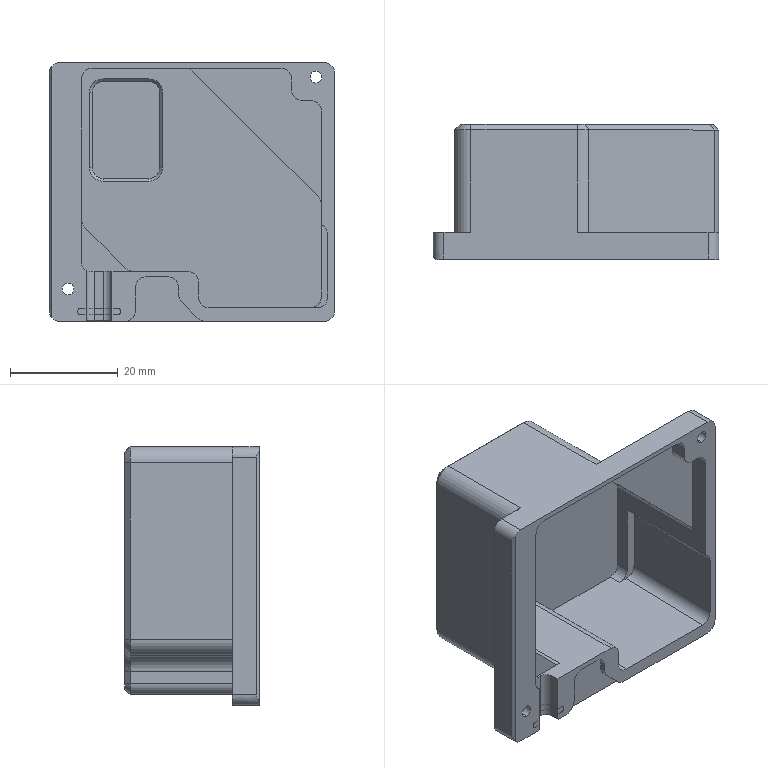Part | 2 solids | 274 faces | box 53 x 25 x 48 mm | volume 26879 mm3 | plane 140 | cylinder 106 | cone 26 | spline 2 | commonest cylinder face diameters 4 x54 3 x20 6 x10 2.2 x8 4.4 x8 1 x4